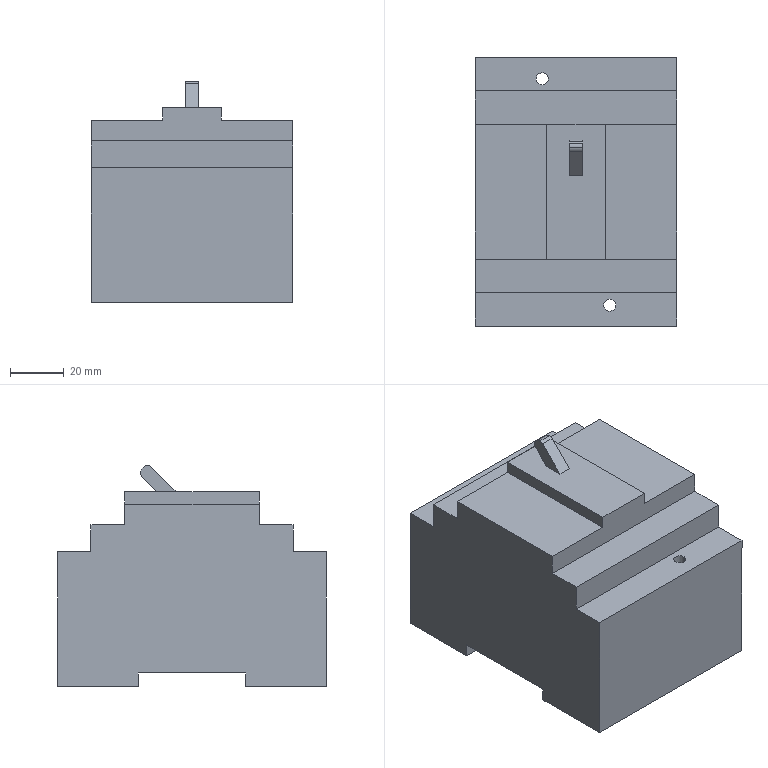Part | SolidWorks | features ICE 5, Extrusion 1, Fillet 1, HoleWzd 1 | 1 solid | 34 faces | box 74.7 x 99.6 x 82.007 mm | volume 445552 mm3 | plane 27 | cylinder 7 | commonest cylinder face diameters 4.5 x4 4 x3
STEP:
#1=CARTESIAN_POINT('',(2.5,16.464,48.157));
#2=VERTEX_POINT('',#1);
#3=CARTESIAN_POINT('',(2.5,15.05,47.571));
#4=VERTEX_POINT('',#3);
#5=CARTESIAN_POINT('',(2.5,16.464,46.157));
#6=DIRECTION('',(1.,0.,0.));
#7=DIRECTION('',(0.,0.,-1.));
#8=AXIS2_PLACEMENT_3D('',#5,#6,#7);
#9=CIRCLE('',#8,2.);
#10=EDGE_CURVE('',#2,#4,#9,.T.);
#11=ORIENTED_EDGE('',*,*,#10,.F.);
#12=CARTESIAN_POINT('',(-2.5,16.464,48.157));
#13=VERTEX_POINT('',#12);
#14=CARTESIAN_POINT('',(2.5,16.464,48.157));
#15=DIRECTION('',(-1.,0.,0.));
#16=VECTOR('',#15,1000.);
#17=LINE('',#14,#16);
#18=EDGE_CURVE('',#2,#13,#17,.T.);
#19=ORIENTED_EDGE('',*,*,#18,.T.);
#20=CARTESIAN_POINT('',(-2.5,15.05,47.571));
#21=VERTEX_POINT('',#20);
#22=CARTESIAN_POINT('',(-2.5,16.464,46.157));
#23=DIRECTION('',(-1.,0.,0.));
#24=DIRECTION('',(0.,0.,-1.));
#25=AXIS2_PLACEMENT_3D('',#22,#23,#24);
#26=CIRCLE('',#25,2.);
#27=EDGE_CURVE('',#21,#13,#26,.T.);
#28=ORIENTED_EDGE('',*,*,#27,.F.);
#29=CARTESIAN_POINT('',(2.5,15.05,47.571));
#30=DIRECTION('',(-1.,0.,0.));
#31=VECTOR('',#30,1000.);
#32=LINE('',#29,#31);
#33=EDGE_CURVE('',#4,#21,#32,.T.);
#34=ORIENTED_EDGE('',*,*,#33,.F.);
#35=EDGE_LOOP('',(#11,#19,#28,#34));
#36=FACE_OUTER_BOUND('',#35,.T.);
#37=CARTESIAN_POINT('',(2.5,16.464,46.157));
#38=DIRECTION('',(-1.,0.,0.));
#39=DIRECTION('',(0.,0.,1.));
#40=AXIS2_PLACEMENT_3D('',#37,#38,#39);
#41=CYLINDRICAL_SURFACE('',#40,2.);
#42=ADVANCED_FACE('',(#36),#41,.T.);
#43=CARTESIAN_POINT('',(-14.75,42.,-33.85));
#44=VERTEX_POINT('',#43);
#45=CARTESIAN_POINT('',(-10.25,42.,-33.85));
#46=VERTEX_POINT('',#45);
#47=CARTESIAN_POINT('',(-12.5,42.,-33.85));
#48=DIRECTION('',(0.,0.,1.));
#49=DIRECTION('',(1.,0.,0.));
#50=AXIS2_PLACEMENT_3D('',#47,#48,#49);
#51=CIRCLE('',#50,2.25);
#52=EDGE_CURVE('',#44,#46,#51,.T.);
#53=ORIENTED_EDGE('',*,*,#52,.F.);
#54=CARTESIAN_POINT('',(-14.75,42.,16.15));
#55=VERTEX_POINT('',#54);
#56=CARTESIAN_POINT('',(-14.75,42.,33.85));
#57=DIRECTION('',(0.,0.,1.));
#58=VECTOR('',#57,1000.);
#59=LINE('',#56,#58);
#60=EDGE_CURVE('',#44,#55,#59,.T.);
#61=ORIENTED_EDGE('',*,*,#60,.T.);
#62=CARTESIAN_POINT('',(-10.25,42.,16.15));
#63=VERTEX_POINT('',#62);
#64=CARTESIAN_POINT('',(-12.5,42.,16.15));
#65=DIRECTION('',(0.,0.,-1.));
#66=DIRECTION('',(1.,0.,0.));
#67=AXIS2_PLACEMENT_3D('',#64,#65,#66);
#68=CIRCLE('',#67,2.25);
#69=EDGE_CURVE('',#63,#55,#68,.T.);
#70=ORIENTED_EDGE('',*,*,#69,.F.);
#71=CARTESIAN_POINT('',(-10.25,42.,33.85));
#72=DIRECTION('',(0.,0.,1.));
#73=VECTOR('',#72,1000.);
#74=LINE('',#71,#73);
#75=EDGE_CURVE('',#46,#63,#74,.T.);
#76=ORIENTED_EDGE('',*,*,#75,.F.);
#77=EDGE_LOOP('',(#53,#61,#70,#76));
#78=FACE_OUTER_BOUND('',#77,.T.);
#79=CARTESIAN_POINT('',(-12.5,42.,33.85));
#80=DIRECTION('',(0.,0.,1.));
#81=DIRECTION('',(1.,0.,0.));
#82=AXIS2_PLACEMENT_3D('',#79,#80,#81);
#83=CYLINDRICAL_SURFACE('',#82,2.25);
#84=ADVANCED_FACE('',(#78),#83,.F.);
#85=CARTESIAN_POINT('',(10.25,-42.,-33.85));
#86=VERTEX_POINT('',#85);
#87=CARTESIAN_POINT('',(14.75,-42.,-33.85));
#88=VERTEX_POINT('',#87);
#89=CARTESIAN_POINT('',(12.5,-42.,-33.85));
#90=DIRECTION('',(0.,0.,1.));
#91=DIRECTION('',(1.,0.,0.));
#92=AXIS2_PLACEMENT_3D('',#89,#90,#91);
#93=CIRCLE('',#92,2.25);
#94=EDGE_CURVE('',#86,#88,#93,.T.);
#95=ORIENTED_EDGE('',*,*,#94,.F.);
#96=CARTESIAN_POINT('',(10.25,-42.,16.15));
#97=VERTEX_POINT('',#96);
#98=CARTESIAN_POINT('',(10.25,-42.,33.85));
#99=DIRECTION('',(0.,0.,1.));
#100=VECTOR('',#99,1000.);
#101=LINE('',#98,#100);
#102=EDGE_CURVE('',#86,#97,#101,.T.);
#103=ORIENTED_EDGE('',*,*,#102,.T.);
#104=CARTESIAN_POINT('',(14.75,-42.,16.15));
#105=VERTEX_POINT('',#104);
#106=CARTESIAN_POINT('',(12.5,-42.,16.15));
#107=DIRECTION('',(0.,0.,-1.));
#108=DIRECTION('',(1.,0.,0.));
#109=AXIS2_PLACEMENT_3D('',#106,#107,#108);
#110=CIRCLE('',#109,2.25);
#111=EDGE_CURVE('',#105,#97,#110,.T.);
#112=ORIENTED_EDGE('',*,*,#111,.F.);
#113=CARTESIAN_POINT('',(14.75,-42.,33.85));
#114=DIRECTION('',(0.,0.,1.));
#115=VECTOR('',#114,1000.);
#116=LINE('',#113,#115);
#117=EDGE_CURVE('',#88,#105,#116,.T.);
#118=ORIENTED_EDGE('',*,*,#117,.F.);
#119=EDGE_LOOP('',(#95,#103,#112,#118));
#120=FACE_OUTER_BOUND('',#119,.T.);
#121=CARTESIAN_POINT('',(12.5,-42.,33.85));
#122=DIRECTION('',(0.,0.,1.));
#123=DIRECTION('',(1.,0.,0.));
#124=AXIS2_PLACEMENT_3D('',#121,#122,#123);
#125=CYLINDRICAL_SURFACE('',#124,2.25);
#126=ADVANCED_FACE('',(#120),#125,.F.);
#127=CARTESIAN_POINT('',(12.5,-42.,-33.85));
#128=DIRECTION('',(0.,0.,1.));
#129=DIRECTION('',(1.,0.,0.));
#130=AXIS2_PLACEMENT_3D('',#127,#128,#129);
#131=CIRCLE('',#130,2.25);
#132=EDGE_CURVE('',#88,#86,#131,.T.);
#133=ORIENTED_EDGE('',*,*,#132,.T.);
#134=ORIENTED_EDGE('',*,*,#94,.T.);
#135=EDGE_LOOP('',(#133,#134));
#136=FACE_BOUND('',#135,.T.);
#137=CARTESIAN_POINT('',(-37.35,-20.,-33.85));
#138=VERTEX_POINT('',#137);
#139=CARTESIAN_POINT('',(-37.35,-49.8,-33.85));
#140=VERTEX_POINT('',#139);
#141=CARTESIAN_POINT('',(-37.35,49.8,-33.85));
#142=DIRECTION('',(0.,-1.,0.));
#143=VECTOR('',#142,1000.);
#144=LINE('',#141,#143);
#145=EDGE_CURVE('',#138,#140,#144,.T.);
#146=ORIENTED_EDGE('',*,*,#145,.F.);
#147=CARTESIAN_POINT('',(37.35,-20.,-33.85));
#148=VERTEX_POINT('',#147);
#149=CARTESIAN_POINT('',(37.35,-20.,-33.85));
#150=DIRECTION('',(1.,0.,0.));
#151=VECTOR('',#150,1000.);
#152=LINE('',#149,#151);
#153=EDGE_CURVE('',#138,#148,#152,.T.);
#154=ORIENTED_EDGE('',*,*,#153,.T.);
#155=CARTESIAN_POINT('',(37.35,-49.8,-33.85));
#156=VERTEX_POINT('',#155);
#157=CARTESIAN_POINT('',(37.35,49.8,-33.85));
#158=DIRECTION('',(0.,1.,0.));
#159=VECTOR('',#158,1000.);
#160=LINE('',#157,#159);
#161=EDGE_CURVE('',#156,#148,#160,.T.);
#162=ORIENTED_EDGE('',*,*,#161,.F.);
#163=CARTESIAN_POINT('',(-37.35,-49.8,-33.85));
#164=DIRECTION('',(1.,0.,0.));
#165=VECTOR('',#164,1000.);
#166=LINE('',#163,#165);
#167=EDGE_CURVE('',#140,#156,#166,.T.);
#168=ORIENTED_EDGE('',*,*,#167,.F.);
#169=EDGE_LOOP('',(#146,#154,#162,#168));
#170=FACE_OUTER_BOUND('',#169,.T.);
#171=CARTESIAN_POINT('',(37.35,-49.8,-33.85));
#172=DIRECTION('',(0.,0.,1.));
#173=DIRECTION('',(1.,0.,0.));
#174=AXIS2_PLACEMENT_3D('',#171,#172,#173);
#175=PLANE('',#174);
#176=ADVANCED_FACE('',(#136,#170),#175,.F.);
#177=CARTESIAN_POINT('',(10.85,-25.,33.85));
#178=VERTEX_POINT('',#177);
#179=CARTESIAN_POINT('',(10.85,25.,33.85));
#180=VERTEX_POINT('',#179);
#181=CARTESIAN_POINT('',(10.85,-25.,33.85));
#182=DIRECTION('',(0.,1.,0.));
#183=VECTOR('',#182,1000.);
#184=LINE('',#181,#183);
#185=EDGE_CURVE('',#178,#180,#184,.T.);
#186=ORIENTED_EDGE('',*,*,#185,.F.);
#187=CARTESIAN_POINT('',(37.35,-25.,33.85));
#188=VERTEX_POINT('',#187);
#189=CARTESIAN_POINT('',(-37.35,-25.,33.85));
#190=DIRECTION('',(-1.,0.,0.));
#191=VECTOR('',#190,1000.);
#192=LINE('',#189,#191);
#193=EDGE_CURVE('',#188,#178,#192,.T.);
#194=ORIENTED_EDGE('',*,*,#193,.F.);
#195=CARTESIAN_POINT('',(37.35,25.,33.85));
#196=VERTEX_POINT('',#195);
#197=CARTESIAN_POINT('',(37.35,49.8,33.85));
#198=DIRECTION('',(0.,1.,0.));
#199=VECTOR('',#198,1000.);
#200=LINE('',#197,#199);
#201=EDGE_CURVE('',#188,#196,#200,.T.);
#202=ORIENTED_EDGE('',*,*,#201,.T.);
#203=CARTESIAN_POINT('',(-37.35,25.,33.85));
#204=DIRECTION('',(1.,0.,0.));
#205=VECTOR('',#204,1000.);
#206=LINE('',#203,#205);
#207=EDGE_CURVE('',#180,#196,#206,.T.);
#208=ORIENTED_EDGE('',*,*,#207,.F.);
#209=EDGE_LOOP('',(#186,#194,#202,#208));
#210=FACE_OUTER_BOUND('',#209,.T.);
#211=CARTESIAN_POINT('',(37.35,-49.8,33.85));
#212=DIRECTION('',(0.,0.,1.));
#213=DIRECTION('',(1.,0.,0.));
#214=AXIS2_PLACEMENT_3D('',#211,#212,#213);
#215=PLANE('',#214);
#216=ADVANCED_FACE('',(#210),#215,.T.);
#217=CARTESIAN_POINT('',(-37.35,-49.8,16.15));
#218=VERTEX_POINT('',#217);
#219=CARTESIAN_POINT('',(37.35,-49.8,16.15));
#220=VERTEX_POINT('',#219);
#221=CARTESIAN_POINT('',(-37.35,-49.8,16.15));
#222=DIRECTION('',(1.,0.,0.));
#223=VECTOR('',#222,1000.);
#224=LINE('',#221,#223);
#225=EDGE_CURVE('',#218,#220,#224,.T.);
#226=ORIENTED_EDGE('',*,*,#225,.F.);
#227=CARTESIAN_POINT('',(-37.35,-49.8,33.85));
#228=DIRECTION('',(0.,0.,-1.));
#229=VECTOR('',#228,1000.);
#230=LINE('',#227,#229);
#231=EDGE_CURVE('',#218,#140,#230,.T.);
#232=ORIENTED_EDGE('',*,*,#231,.T.);
#233=ORIENTED_EDGE('',*,*,#167,.T.);
#234=CARTESIAN_POINT('',(37.35,-49.8,33.85));
#235=DIRECTION('',(0.,0.,-1.));
#236=VECTOR('',#235,1000.);
#237=LINE('',#234,#236);
#238=EDGE_CURVE('',#220,#156,#237,.T.);
#239=ORIENTED_EDGE('',*,*,#238,.F.);
#240=EDGE_LOOP('',(#226,#232,#233,#239));
#241=FACE_OUTER_BOUND('',#240,.T.);
#242=CARTESIAN_POINT('',(-37.35,-49.8,33.85));
#243=DIRECTION('',(0.,1.,0.));
#244=DIRECTION('',(0.,0.,1.));
#245=AXIS2_PLACEMENT_3D('',#242,#243,#244);
#246=PLANE('',#245);
#247=ADVANCED_FACE('',(#241),#246,.F.);
#248=ORIENTED_EDGE('',*,*,#102,.F.);
#249=ORIENTED_EDGE('',*,*,#132,.F.);
#250=ORIENTED_EDGE('',*,*,#117,.T.);
#251=CARTESIAN_POINT('',(12.5,-42.,16.15));
#252=DIRECTION('',(0.,0.,-1.));
#253=DIRECTION('',(1.,0.,0.));
#254=AXIS2_PLACEMENT_3D('',#251,#252,#253);
#255=CIRCLE('',#254,2.25);
#256=EDGE_CURVE('',#97,#105,#255,.T.);
#257=ORIENTED_EDGE('',*,*,#256,.F.);
#258=EDGE_LOOP('',(#248,#249,#250,#257));
#259=FACE_OUTER_BOUND('',#258,.T.);
#260=CARTESIAN_POINT('',(12.5,-42.,33.85));
#261=DIRECTION('',(0.,0.,1.));
#262=DIRECTION('',(1.,0.,0.));
#263=AXIS2_PLACEMENT_3D('',#260,#261,#262);
#264=CYLINDRICAL_SURFACE('',#263,2.25);
#265=ADVANCED_FACE('',(#259),#264,.F.);
#266=CARTESIAN_POINT('',(37.35,49.8,16.15));
#267=VERTEX_POINT('',#266);
#268=CARTESIAN_POINT('',(-37.35,49.8,16.15));
#269=VERTEX_POINT('',#268);
#270=CARTESIAN_POINT('',(-37.35,49.8,16.15));
#271=DIRECTION('',(-1.,0.,0.));
#272=VECTOR('',#271,1000.);
#273=LINE('',#270,#272);
#274=EDGE_CURVE('',#267,#269,#273,.T.);
#275=ORIENTED_EDGE('',*,*,#274,.F.);
#276=CARTESIAN_POINT('',(37.35,49.8,-33.85));
#277=VERTEX_POINT('',#276);
#278=CARTESIAN_POINT('',(37.35,49.8,33.85));
#279=DIRECTION('',(0.,0.,-1.));
#280=VECTOR('',#279,1000.);
#281=LINE('',#278,#280);
#282=EDGE_CURVE('',#267,#277,#281,.T.);
#283=ORIENTED_EDGE('',*,*,#282,.T.);
#284=CARTESIAN_POINT('',(-37.35,49.8,-33.85));
#285=VERTEX_POINT('',#284);
#286=CARTESIAN_POINT('',(-37.35,49.8,-33.85));
#287=DIRECTION('',(-1.,0.,0.));
#288=VECTOR('',#287,1000.);
#289=LINE('',#286,#288);
#290=EDGE_CURVE('',#277,#285,#289,.T.);
#291=ORIENTED_EDGE('',*,*,#290,.T.);
#292=CARTESIAN_POINT('',(-37.35,49.8,33.85));
#293=DIRECTION('',(0.,0.,-1.));
#294=VECTOR('',#293,1000.);
#295=LINE('',#292,#294);
#296=EDGE_CURVE('',#269,#285,#295,.T.);
#297=ORIENTED_EDGE('',*,*,#296,.F.);
#298=EDGE_LOOP('',(#275,#283,#291,#297));
#299=FACE_OUTER_BOUND('',#298,.T.);
#300=CARTESIAN_POINT('',(-37.35,49.8,33.85));
#301=DIRECTION('',(0.,-1.,0.));
#302=DIRECTION('',(0.,0.,-1.));
#303=AXIS2_PLACEMENT_3D('',#300,#301,#302);
#304=PLANE('',#303);
#305=ADVANCED_FACE('',(#299),#304,.F.);
#306=ORIENTED_EDGE('',*,*,#60,.F.);
#307=CARTESIAN_POINT('',(-12.5,42.,-33.85));
#308=DIRECTION('',(0.,0.,1.));
#309=DIRECTION('',(1.,0.,0.));
#310=AXIS2_PLACEMENT_3D('',#307,#308,#309);
#311=CIRCLE('',#310,2.25);
#312=EDGE_CURVE('',#46,#44,#311,.T.);
#313=ORIENTED_EDGE('',*,*,#312,.F.);
#314=ORIENTED_EDGE('',*,*,#75,.T.);
#315=CARTESIAN_POINT('',(-12.5,42.,16.15));
#316=DIRECTION('',(0.,0.,-1.));
#317=DIRECTION('',(1.,0.,0.));
#318=AXIS2_PLACEMENT_3D('',#315,#316,#317);
#319=CIRCLE('',#318,2.25);
#320=EDGE_CURVE('',#55,#63,#319,.T.);
#321=ORIENTED_EDGE('',*,*,#320,.F.);
#322=EDGE_LOOP('',(#306,#313,#314,#321));
#323=FACE_OUTER_BOUND('',#322,.T.);
#324=CARTESIAN_POINT('',(-12.5,42.,33.85));
#325=DIRECTION('',(0.,0.,1.));
#326=DIRECTION('',(1.,0.,0.));
#327=AXIS2_PLACEMENT_3D('',#324,#325,#326);
#328=CYLINDRICAL_SURFACE('',#327,2.25);
#329=ADVANCED_FACE('',(#323),#328,.F.);
#330=ORIENTED_EDGE('',*,*,#161,.T.);
#331=CARTESIAN_POINT('',(37.35,-20.,-28.85));
#332=VERTEX_POINT('',#331);
#333=CARTESIAN_POINT('',(37.35,-20.,-33.85));
#334=DIRECTION('',(0.,0.,-1.));
#335=VECTOR('',#334,1000.);
#336=LINE('',#333,#335);
#337=EDGE_CURVE('',#332,#148,#336,.T.);
#338=ORIENTED_EDGE('',*,*,#337,.F.);
#339=CARTESIAN_POINT('',(37.35,20.,-28.85));
#340=VERTEX_POINT('',#339);
#341=CARTESIAN_POINT('',(37.35,-20.,-28.85));
#342=DIRECTION('',(0.,-1.,0.));
#343=VECTOR('',#342,1000.);
#344=LINE('',#341,#343);
#345=EDGE_CURVE('',#340,#332,#344,.T.);
#346=ORIENTED_EDGE('',*,*,#345,.F.);
#347=CARTESIAN_POINT('',(37.35,20.,-33.85));
#348=VERTEX_POINT('',#347);
#349=CARTESIAN_POINT('',(37.35,20.,-33.85));
#350=DIRECTION('',(0.,0.,1.));
#351=VECTOR('',#350,1000.);
#352=LINE('',#349,#351);
#353=EDGE_CURVE('',#348,#340,#352,.T.);
#354=ORIENTED_EDGE('',*,*,#353,.F.);
#355=CARTESIAN_POINT('',(37.35,49.8,-33.85));
#356=DIRECTION('',(0.,1.,0.));
#357=VECTOR('',#356,1000.);
#358=LINE('',#355,#357);
#359=EDGE_CURVE('',#348,#277,#358,.T.);
#360=ORIENTED_EDGE('',*,*,#359,.T.);
#361=ORIENTED_EDGE('',*,*,#282,.F.);
#362=CARTESIAN_POINT('',(37.35,37.5,16.15));
#363=VERTEX_POINT('',#362);
#364=CARTESIAN_POINT('',(37.35,49.8,16.15));
#365=DIRECTION('',(0.,1.,0.));
#366=VECTOR('',#365,1000.);
#367=LINE('',#364,#366);
#368=EDGE_CURVE('',#363,#267,#367,.T.);
#369=ORIENTED_EDGE('',*,*,#368,.F.);
#370=CARTESIAN_POINT('',(37.35,37.5,26.15));
#371=VERTEX_POINT('',#370);
#372=CARTESIAN_POINT('',(37.35,37.5,16.15));
#373=DIRECTION('',(0.,0.,1.));
#374=VECTOR('',#373,1000.);
#375=LINE('',#372,#374);
#376=EDGE_CURVE('',#363,#371,#375,.T.);
#377=ORIENTED_EDGE('',*,*,#376,.T.);
#378=CARTESIAN_POINT('',(37.35,25.,26.15));
#379=VERTEX_POINT('',#378);
#380=CARTESIAN_POINT('',(37.35,37.5,26.15));
#381=DIRECTION('',(0.,1.,0.));
#382=VECTOR('',#381,1000.);
#383=LINE('',#380,#382);
#384=EDGE_CURVE('',#379,#371,#383,.T.);
#385=ORIENTED_EDGE('',*,*,#384,.F.);
#386=CARTESIAN_POINT('',(37.35,25.,26.15));
#387=DIRECTION('',(0.,0.,1.));
#388=VECTOR('',#387,1000.);
#389=LINE('',#386,#388);
#390=EDGE_CURVE('',#379,#196,#389,.T.);
#391=ORIENTED_EDGE('',*,*,#390,.T.);
#392=ORIENTED_EDGE('',*,*,#201,.F.);
#393=CARTESIAN_POINT('',(37.35,-25.,26.15));
#394=VERTEX_POINT('',#393);
#395=CARTESIAN_POINT('',(37.35,-25.,26.15));
#396=DIRECTION('',(0.,0.,1.));
#397=VECTOR('',#396,1000.);
#398=LINE('',#395,#397);
#399=EDGE_CURVE('',#394,#188,#398,.T.);
#400=ORIENTED_EDGE('',*,*,#399,.F.);
#401=CARTESIAN_POINT('',(37.35,-37.5,26.15));
#402=VERTEX_POINT('',#401);
#403=CARTESIAN_POINT('',(37.35,-37.5,26.15));
#404=DIRECTION('',(0.,1.,0.));
#405=VECTOR('',#404,1000.);
#406=LINE('',#403,#405);
#407=EDGE_CURVE('',#402,#394,#406,.T.);
#408=ORIENTED_EDGE('',*,*,#407,.F.);
#409=CARTESIAN_POINT('',(37.35,-37.5,16.15));
#410=VERTEX_POINT('',#409);
#411=CARTESIAN_POINT('',(37.35,-37.5,16.15));
#412=DIRECTION('',(0.,0.,1.));
#413=VECTOR('',#412,1000.);
#414=LINE('',#411,#413);
#415=EDGE_CURVE('',#410,#402,#414,.T.);
#416=ORIENTED_EDGE('',*,*,#415,.F.);
#417=CARTESIAN_POINT('',(37.35,-49.8,16.15));
#418=DIRECTION('',(0.,1.,0.));
#419=VECTOR('',#418,1000.);
#420=LINE('',#417,#419);
#421=EDGE_CURVE('',#220,#410,#420,.T.);
#422=ORIENTED_EDGE('',*,*,#421,.F.);
#423=ORIENTED_EDGE('',*,*,#238,.T.);
#424=EDGE_LOOP('',(#330,#338,#346,#354,#360,#361,#369,#377,#385,#391,#392,#400,#408,#416,#422,#423));
#425=FACE_OUTER_BOUND('',#424,.T.);
#426=CARTESIAN_POINT('',(37.35,49.8,33.85));
#427=DIRECTION('',(-1.,0.,0.));
#428=DIRECTION('',(0.,-1.,0.));
#429=AXIS2_PLACEMENT_3D('',#426,#427,#428);
#430=PLANE('',#429);
#431=ADVANCED_FACE('',(#425),#430,.F.);
#432=CARTESIAN_POINT('',(-37.35,20.,-28.85));
#433=VERTEX_POINT('',#432);
#434=CARTESIAN_POINT('',(-37.35,-20.,-28.85));
#435=VERTEX_POINT('',#434);
#436=CARTESIAN_POINT('',(-37.35,49.8,-28.85));
#437=DIRECTION('',(0.,-1.,0.));
#438=VECTOR('',#437,1000.);
#439=LINE('',#436,#438);
#440=EDGE_CURVE('',#433,#435,#439,.T.);
#441=ORIENTED_EDGE('',*,*,#440,.T.);
#442=CARTESIAN_POINT('',(-37.35,-20.,33.85));
#443=DIRECTION('',(0.,0.,-1.));
#444=VECTOR('',#443,1000.);
#445=LINE('',#442,#444);
#446=EDGE_CURVE('',#435,#138,#445,.T.);
#447=ORIENTED_EDGE('',*,*,#446,.T.);
#448=ORIENTED_EDGE('',*,*,#145,.T.);
#449=ORIENTED_EDGE('',*,*,#231,.F.);
#450=CARTESIAN_POINT('',(-37.35,-37.5,16.15));
#451=VERTEX_POINT('',#450);
#452=CARTESIAN_POINT('',(-37.35,-49.8,16.15));
#453=DIRECTION('',(0.,-1.,0.));
#454=VECTOR('',#453,1000.);
#455=LINE('',#452,#454);
#456=EDGE_CURVE('',#451,#218,#455,.T.);
#457=ORIENTED_EDGE('',*,*,#456,.F.);
#458=CARTESIAN_POINT('',(-37.35,-37.5,26.15));
#459=VERTEX_POINT('',#458);
#460=CARTESIAN_POINT('',(-37.35,-37.5,16.15));
#461=DIRECTION('',(0.,0.,1.));
#462=VECTOR('',#461,1000.);
#463=LINE('',#460,#462);
#464=EDGE_CURVE('',#451,#459,#463,.T.);
#465=ORIENTED_EDGE('',*,*,#464,.T.);
#466=CARTESIAN_POINT('',(-37.35,-25.,26.15));
#467=VERTEX_POINT('',#466);
#468=CARTESIAN_POINT('',(-37.35,-37.5,26.15));
#469=DIRECTION('',(0.,-1.,0.));
#470=VECTOR('',#469,1000.);
#471=LINE('',#468,#470);
#472=EDGE_CURVE('',#467,#459,#471,.T.);
#473=ORIENTED_EDGE('',*,*,#472,.F.);
#474=CARTESIAN_POINT('',(-37.35,-25.,33.85));
#475=VERTEX_POINT('',#474);
#476=CARTESIAN_POINT('',(-37.35,-25.,26.15));
#477=DIRECTION('',(0.,0.,1.));
#478=VECTOR('',#477,1000.);
#479=LINE('',#476,#478);
#480=EDGE_CURVE('',#467,#475,#479,.T.);
#481=ORIENTED_EDGE('',*,*,#480,.T.);
#482=CARTESIAN_POINT('',(-37.35,25.,33.85));
#483=VERTEX_POINT('',#482);
#484=CARTESIAN_POINT('',(-37.35,49.8,33.85));
#485=DIRECTION('',(0.,-1.,0.));
#486=VECTOR('',#485,1000.);
#487=LINE('',#484,#486);
#488=EDGE_CURVE('',#483,#475,#487,.T.);
#489=ORIENTED_EDGE('',*,*,#488,.F.);
#490=CARTESIAN_POINT('',(-37.35,25.,26.15));
#491=VERTEX_POINT('',#490);
#492=CARTESIAN_POINT('',(-37.35,25.,26.15));
#493=DIRECTION('',(0.,0.,1.));
#494=VECTOR('',#493,1000.);
#495=LINE('',#492,#494);
#496=EDGE_CURVE('',#491,#483,#495,.T.);
#497=ORIENTED_EDGE('',*,*,#496,.F.);
#498=CARTESIAN_POINT('',(-37.35,37.5,26.15));
#499=VERTEX_POINT('',#498);
#500=CARTESIAN_POINT('',(-37.35,37.5,26.15));
#501=DIRECTION('',(0.,-1.,0.));
#502=VECTOR('',#501,1000.);
#503=LINE('',#500,#502);
#504=EDGE_CURVE('',#499,#491,#503,.T.);
#505=ORIENTED_EDGE('',*,*,#504,.F.);
#506=CARTESIAN_POINT('',(-37.35,37.5,16.15));
#507=VERTEX_POINT('',#506);
#508=CARTESIAN_POINT('',(-37.35,37.5,16.15));
#509=DIRECTION('',(0.,0.,1.));
#510=VECTOR('',#509,1000.);
#511=LINE('',#508,#510);
#512=EDGE_CURVE('',#507,#499,#511,.T.);
#513=ORIENTED_EDGE('',*,*,#512,.F.);
#514=CARTESIAN_POINT('',(-37.35,49.8,16.15));
#515=DIRECTION('',(0.,-1.,0.));
#516=VECTOR('',#515,1000.);
#517=LINE('',#514,#516);
#518=EDGE_CURVE('',#269,#507,#517,.T.);
#519=ORIENTED_EDGE('',*,*,#518,.F.);
#520=ORIENTED_EDGE('',*,*,#296,.T.);
#521=CARTESIAN_POINT('',(-37.35,20.,-33.85));
#522=VERTEX_POINT('',#521);
#523=CARTESIAN_POINT('',(-37.35,49.8,-33.85));
#524=DIRECTION('',(0.,-1.,0.));
#525=VECTOR('',#524,1000.);
#526=LINE('',#523,#525);
#527=EDGE_CURVE('',#285,#522,#526,.T.);
#528=ORIENTED_EDGE('',*,*,#527,.T.);
#529=CARTESIAN_POINT('',(-37.35,20.,33.85));
#530=DIRECTION('',(0.,0.,1.));
#531=VECTOR('',#530,1000.);
#532=LINE('',#529,#531);
#533=EDGE_CURVE('',#522,#433,#532,.T.);
#534=ORIENTED_EDGE('',*,*,#533,.T.);
#535=EDGE_LOOP('',(#441,#447,#448,#449,#457,#465,#473,#481,#489,#497,#505,#513,#519,#520,#528,#534));
#536=FACE_OUTER_BOUND('',#535,.T.);
#537=CARTESIAN_POINT('',(-37.35,49.8,33.85));
#538=DIRECTION('',(1.,0.,0.));
#539=DIRECTION('',(0.,1.,0.));
#540=AXIS2_PLACEMENT_3D('',#537,#538,#539);
#541=PLANE('',#540);
#542=ADVANCED_FACE('',(#536),#541,.F.);
#543=CARTESIAN_POINT('',(-10.85,25.,33.85));
#544=VERTEX_POINT('',#543);
#545=CARTESIAN_POINT('',(-10.85,-25.,33.85));
#546=VERTEX_POINT('',#545);
#547=CARTESIAN_POINT('',(-10.85,-25.,33.85));
#548=DIRECTION('',(0.,-1.,0.));
#549=VECTOR('',#548,1000.);
#550=LINE('',#547,#549);
#551=EDGE_CURVE('',#544,#546,#550,.T.);
#552=ORIENTED_EDGE('',*,*,#551,.F.);
#553=CARTESIAN_POINT('',(-37.35,25.,33.85));
#554=DIRECTION('',(1.,0.,0.));
#555=VECTOR('',#554,1000.);
#556=LINE('',#553,#555);
#557=EDGE_CURVE('',#483,#544,#556,.T.);
#558=ORIENTED_EDGE('',*,*,#557,.F.);
#559=ORIENTED_EDGE('',*,*,#488,.T.);
#560=CARTESIAN_POINT('',(-37.35,-25.,33.85));
#561=DIRECTION('',(-1.,0.,0.));
#562=VECTOR('',#561,1000.);
#563=LINE('',#560,#562);
#564=EDGE_CURVE('',#546,#475,#563,.T.);
#565=ORIENTED_EDGE('',*,*,#564,.F.);
#566=EDGE_LOOP('',(#552,#558,#559,#565));
#567=FACE_OUTER_BOUND('',#566,.T.);
#568=CARTESIAN_POINT('',(37.35,-49.8,33.85));
#569=DIRECTION('',(0.,0.,1.));
#570=DIRECTION('',(1.,0.,0.));
#571=AXIS2_PLACEMENT_3D('',#568,#569,#570);
#572=PLANE('',#571);
#573=ADVANCED_FACE('',(#567),#572,.T.);
#574=ORIENTED_EDGE('',*,*,#312,.T.);
#575=ORIENTED_EDGE('',*,*,#52,.T.);
#576=EDGE_LOOP('',(#574,#575));
#577=FACE_BOUND('',#576,.T.);
#578=ORIENTED_EDGE('',*,*,#359,.F.);
#579=CARTESIAN_POINT('',(37.35,20.,-33.85));
#580=DIRECTION('',(-1.,0.,0.));
#581=VECTOR('',#580,1000.);
#582=LINE('',#579,#581);
#583=EDGE_CURVE('',#348,#522,#582,.T.);
#584=ORIENTED_EDGE('',*,*,#583,.T.);
#585=ORIENTED_EDGE('',*,*,#527,.F.);
#586=ORIENTED_EDGE('',*,*,#290,.F.);
#587=EDGE_LOOP('',(#578,#584,#585,#586));
#588=FACE_OUTER_BOUND('',#587,.T.);
#589=CARTESIAN_POINT('',(37.35,-49.8,-33.85));
#590=DIRECTION('',(0.,0.,1.));
#591=DIRECTION('',(1.,0.,0.));
#592=AXIS2_PLACEMENT_3D('',#589,#590,#591);
#593=PLANE('',#592);
#594=ADVANCED_FACE('',(#577,#588),#593,.F.);
#595=ORIENTED_EDGE('',*,*,#518,.T.);
#596=CARTESIAN_POINT('',(-37.35,37.5,16.15));
#597=DIRECTION('',(1.,0.,0.));
#598=VECTOR('',#597,1000.);
#599=LINE('',#596,#598);
#600=EDGE_CURVE('',#507,#363,#599,.T.);
#601=ORIENTED_EDGE('',*,*,#600,.T.);
#602=ORIENTED_EDGE('',*,*,#368,.T.);
#603=ORIENTED_EDGE('',*,*,#274,.T.);
#604=EDGE_LOOP('',(#595,#601,#602,#603));
#605=FACE_OUTER_BOUND('',#604,.T.);
#606=ORIENTED_EDGE('',*,*,#69,.T.);
#607=ORIENTED_EDGE('',*,*,#320,.T.);
#608=EDGE_LOOP('',(#606,#607));
#609=FACE_BOUND('',#608,.T.);
#610=CARTESIAN_POINT('',(-37.35,37.5,16.15));
#611=DIRECTION('',(0.,0.,1.));
#612=DIRECTION('',(1.,0.,0.));
#613=AXIS2_PLACEMENT_3D('',#610,#611,#612);
#614=PLANE('',#613);
#615=ADVANCED_FACE('',(#605,#609),#614,.T.);
#616=ORIENTED_EDGE('',*,*,#512,.T.);
#617=CARTESIAN_POINT('',(-37.35,37.5,26.15));
#618=DIRECTION('',(-1.,0.,0.));
#619=VECTOR('',#618,1000.);
#620=LINE('',#617,#619);
#621=EDGE_CURVE('',#371,#499,#620,.T.);
#622=ORIENTED_EDGE('',*,*,#621,.F.);
#623=ORIENTED_EDGE('',*,*,#376,.F.);
#624=ORIENTED_EDGE('',*,*,#600,.F.);
#625=EDGE_LOOP('',(#616,#622,#623,#624));
#626=FACE_OUTER_BOUND('',#625,.T.);
#627=CARTESIAN_POINT('',(-37.35,37.5,16.15));
#628=DIRECTION('',(0.,-1.,0.));
#629=DIRECTION('',(0.,0.,-1.));
#630=AXIS2_PLACEMENT_3D('',#627,#628,#629);
#631=PLANE('',#630);
#632=ADVANCED_FACE('',(#626),#631,.F.);
#633=ORIENTED_EDGE('',*,*,#225,.T.);
#634=ORIENTED_EDGE('',*,*,#421,.T.);
#635=CARTESIAN_POINT('',(-37.35,-37.5,16.15));
#636=DIRECTION('',(-1.,0.,0.));
#637=VECTOR('',#636,1000.);
#638=LINE('',#635,#637);
#639=EDGE_CURVE('',#410,#451,#638,.T.);
#640=ORIENTED_EDGE('',*,*,#639,.T.);
#641=ORIENTED_EDGE('',*,*,#456,.T.);
#642=EDGE_LOOP('',(#633,#634,#640,#641));
#643=FACE_OUTER_BOUND('',#642,.T.);
#644=ORIENTED_EDGE('',*,*,#111,.T.);
#645=ORIENTED_EDGE('',*,*,#256,.T.);
#646=EDGE_LOOP('',(#644,#645));
#647=FACE_BOUND('',#646,.T.);
#648=CARTESIAN_POINT('',(37.35,-49.8,16.15));
#649=DIRECTION('',(0.,0.,1.));
#650=DIRECTION('',(1.,0.,0.));
#651=AXIS2_PLACEMENT_3D('',#648,#649,#650);
#652=PLANE('',#651);
#653=ADVANCED_FACE('',(#643,#647),#652,.T.);
#654=ORIENTED_EDGE('',*,*,#415,.T.);
#655=CARTESIAN_POINT('',(-37.35,-37.5,26.15));
#656=DIRECTION('',(1.,0.,0.));
#657=VECTOR('',#656,1000.);
#658=LINE('',#655,#657);
#659=EDGE_CURVE('',#459,#402,#658,.T.);
#660=ORIENTED_EDGE('',*,*,#659,.F.);
#661=ORIENTED_EDGE('',*,*,#464,.F.);
#662=ORIENTED_EDGE('',*,*,#639,.F.);
#663=EDGE_LOOP('',(#654,#660,#661,#662));
#664=FACE_OUTER_BOUND('',#663,.T.);
#665=CARTESIAN_POINT('',(-37.35,-37.5,16.15));
#666=DIRECTION('',(0.,1.,0.));
#667=DIRECTION('',(0.,0.,1.));
#668=AXIS2_PLACEMENT_3D('',#665,#666,#667);
#669=PLANE('',#668);
#670=ADVANCED_FACE('',(#664),#669,.F.);
#671=ORIENTED_EDGE('',*,*,#193,.T.);
#672=CARTESIAN_POINT('',(10.85,-25.,38.45));
#673=VERTEX_POINT('',#672);
#674=CARTESIAN_POINT('',(10.85,-25.,38.45));
#675=DIRECTION('',(0.,0.,-1.));
#676=VECTOR('',#675,1000.);
#677=LINE('',#674,#676);
#678=EDGE_CURVE('',#673,#178,#677,.T.);
#679=ORIENTED_EDGE('',*,*,#678,.F.);
#680=CARTESIAN_POINT('',(-10.85,-25.,38.45));
#681=VERTEX_POINT('',#680);
#682=CARTESIAN_POINT('',(-10.85,-25.,38.45));
#683=DIRECTION('',(1.,0.,0.));
#684=VECTOR('',#683,1000.);
#685=LINE('',#682,#684);
#686=EDGE_CURVE('',#681,#673,#685,.T.);
#687=ORIENTED_EDGE('',*,*,#686,.F.);
#688=CARTESIAN_POINT('',(-10.85,-25.,38.45));
#689=DIRECTION('',(0.,0.,-1.));
#690=VECTOR('',#689,1000.);
#691=LINE('',#688,#690);
#692=EDGE_CURVE('',#681,#546,#691,.T.);
#693=ORIENTED_EDGE('',*,*,#692,.T.);
#694=ORIENTED_EDGE('',*,*,#564,.T.);
#695=ORIENTED_EDGE('',*,*,#480,.F.);
#696=CARTESIAN_POINT('',(-37.35,-25.,26.15));
#697=DIRECTION('',(-1.,0.,0.));
#698=VECTOR('',#697,1000.);
#699=LINE('',#696,#698);
#700=EDGE_CURVE('',#394,#467,#699,.T.);
#701=ORIENTED_EDGE('',*,*,#700,.F.);
#702=ORIENTED_EDGE('',*,*,#399,.T.);
#703=EDGE_LOOP('',(#671,#679,#687,#693,#694,#695,#701,#702));
#704=FACE_OUTER_BOUND('',#703,.T.);
#705=CARTESIAN_POINT('',(-37.35,-25.,26.15));
#706=DIRECTION('',(0.,1.,0.));
#707=DIRECTION('',(0.,0.,1.));
#708=AXIS2_PLACEMENT_3D('',#705,#706,#707);
#709=PLANE('',#708);
#710=ADVANCED_FACE('',(#704),#709,.F.);
#711=ORIENTED_EDGE('',*,*,#472,.T.);
#712=ORIENTED_EDGE('',*,*,#659,.T.);
#713=ORIENTED_EDGE('',*,*,#407,.T.);
#714=ORIENTED_EDGE('',*,*,#700,.T.);
#715=EDGE_LOOP('',(#711,#712,#713,#714));
#716=FACE_OUTER_BOUND('',#715,.T.);
#717=CARTESIAN_POINT('',(-37.35,-25.,26.15));
#718=DIRECTION('',(0.,0.,-1.));
#719=DIRECTION('',(-1.,0.,0.));
#720=AXIS2_PLACEMENT_3D('',#717,#718,#719);
#721=PLANE('',#720);
#722=ADVANCED_FACE('',(#716),#721,.F.);
#723=ORIENTED_EDGE('',*,*,#557,.T.);
#724=CARTESIAN_POINT('',(-10.85,25.,38.45));
#725=VERTEX_POINT('',#724);
#726=CARTESIAN_POINT('',(-10.85,25.,38.45));
#727=DIRECTION('',(0.,0.,-1.));
#728=VECTOR('',#727,1000.);
#729=LINE('',#726,#728);
#730=EDGE_CURVE('',#725,#544,#729,.T.);
#731=ORIENTED_EDGE('',*,*,#730,.F.);
#732=CARTESIAN_POINT('',(10.85,25.,38.45));
#733=VERTEX_POINT('',#732);
#734=CARTESIAN_POINT('',(-10.85,25.,38.45));
#735=DIRECTION('',(-1.,0.,0.));
#736=VECTOR('',#735,1000.);
#737=LINE('',#734,#736);
#738=EDGE_CURVE('',#733,#725,#737,.T.);
#739=ORIENTED_EDGE('',*,*,#738,.F.);
#740=CARTESIAN_POINT('',(10.85,25.,38.45));
#741=DIRECTION('',(0.,0.,-1.));
#742=VECTOR('',#741,1000.);
#743=LINE('',#740,#742);
#744=EDGE_CURVE('',#733,#180,#743,.T.);
#745=ORIENTED_EDGE('',*,*,#744,.T.);
#746=ORIENTED_EDGE('',*,*,#207,.T.);
#747=ORIENTED_EDGE('',*,*,#390,.F.);
#748=CARTESIAN_POINT('',(-37.35,25.,26.15));
#749=DIRECTION('',(1.,0.,0.));
#750=VECTOR('',#749,1000.);
#751=LINE('',#748,#750);
#752=EDGE_CURVE('',#491,#379,#751,.T.);
#753=ORIENTED_EDGE('',*,*,#752,.F.);
#754=ORIENTED_EDGE('',*,*,#496,.T.);
#755=EDGE_LOOP('',(#723,#731,#739,#745,#746,#747,#753,#754));
#756=FACE_OUTER_BOUND('',#755,.T.);
#757=CARTESIAN_POINT('',(-37.35,25.,26.15));
#758=DIRECTION('',(0.,-1.,0.));
#759=DIRECTION('',(1.,0.,0.));
#760=AXIS2_PLACEMENT_3D('',#757,#758,#759);
#761=PLANE('',#760);
#762=ADVANCED_FACE('',(#756),#761,.F.);
#763=ORIENTED_EDGE('',*,*,#621,.T.);
#764=ORIENTED_EDGE('',*,*,#504,.T.);
#765=ORIENTED_EDGE('',*,*,#752,.T.);
#766=ORIENTED_EDGE('',*,*,#384,.T.);
#767=EDGE_LOOP('',(#763,#764,#765,#766));
#768=FACE_OUTER_BOUND('',#767,.T.);
#769=CARTESIAN_POINT('',(37.35,37.5,26.15));
#770=DIRECTION('',(0.,0.,-1.));
#771=DIRECTION('',(-1.,0.,0.));
#772=AXIS2_PLACEMENT_3D('',#769,#770,#771);
#773=PLANE('',#772);
#774=ADVANCED_FACE('',(#768),#773,.F.);
#775=ORIENTED_EDGE('',*,*,#185,.T.);
#776=ORIENTED_EDGE('',*,*,#744,.F.);
#777=CARTESIAN_POINT('',(10.85,-25.,38.45));
#778=DIRECTION('',(0.,1.,0.));
#779=VECTOR('',#778,1000.);
#780=LINE('',#777,#779);
#781=EDGE_CURVE('',#673,#733,#780,.T.);
#782=ORIENTED_EDGE('',*,*,#781,.F.);
#783=ORIENTED_EDGE('',*,*,#678,.T.);
#784=EDGE_LOOP('',(#775,#776,#782,#783));
#785=FACE_OUTER_BOUND('',#784,.T.);
#786=CARTESIAN_POINT('',(10.85,-25.,38.45));
#787=DIRECTION('',(-1.,0.,0.));
#788=DIRECTION('',(0.,0.,1.));
#789=AXIS2_PLACEMENT_3D('',#786,#787,#788);
#790=PLANE('',#789);
#791=ADVANCED_FACE('',(#785),#790,.F.);
#792=ORIENTED_EDGE('',*,*,#551,.T.);
#793=ORIENTED_EDGE('',*,*,#692,.F.);
#794=CARTESIAN_POINT('',(-10.85,-25.,38.45));
#795=DIRECTION('',(0.,-1.,0.));
#796=VECTOR('',#795,1000.);
#797=LINE('',#794,#796);
#798=EDGE_CURVE('',#725,#681,#797,.T.);
#799=ORIENTED_EDGE('',*,*,#798,.F.);
#800=ORIENTED_EDGE('',*,*,#730,.T.);
#801=EDGE_LOOP('',(#792,#793,#799,#800));
#802=FACE_OUTER_BOUND('',#801,.T.);
#803=CARTESIAN_POINT('',(-10.85,-25.,38.45));
#804=DIRECTION('',(1.,0.,0.));
#805=DIRECTION('',(0.,0.,-1.));
#806=AXIS2_PLACEMENT_3D('',#803,#804,#805);
#807=PLANE('',#806);
#808=ADVANCED_FACE('',(#802),#807,.F.);
#809=CARTESIAN_POINT('',(2.5,13.,38.45));
#810=VERTEX_POINT('',#809);
#811=CARTESIAN_POINT('',(-2.5,13.,38.45));
#812=VERTEX_POINT('',#811);
#813=CARTESIAN_POINT('',(2.5,13.,38.45));
#814=DIRECTION('',(-1.,0.,0.));
#815=VECTOR('',#814,1000.);
#816=LINE('',#813,#815);
#817=EDGE_CURVE('',#810,#812,#816,.T.);
#818=ORIENTED_EDGE('',*,*,#817,.F.);
#819=CARTESIAN_POINT('',(2.5,5.929,38.45));
#820=VERTEX_POINT('',#819);
#821=CARTESIAN_POINT('',(2.5,13.,38.45));
#822=DIRECTION('',(0.,1.,0.));
#823=VECTOR('',#822,1000.);
#824=LINE('',#821,#823);
#825=EDGE_CURVE('',#820,#810,#824,.T.);
#826=ORIENTED_EDGE('',*,*,#825,.F.);
#827=CARTESIAN_POINT('',(-2.5,5.929,38.45));
#828=VERTEX_POINT('',#827);
#829=CARTESIAN_POINT('',(2.5,5.929,38.45));
#830=DIRECTION('',(-1.,0.,0.));
#831=VECTOR('',#830,1000.);
#832=LINE('',#829,#831);
#833=EDGE_CURVE('',#820,#828,#832,.T.);
#834=ORIENTED_EDGE('',*,*,#833,.T.);
#835=CARTESIAN_POINT('',(-2.5,13.,38.45));
#836=DIRECTION('',(0.,1.,0.));
#837=VECTOR('',#836,1000.);
#838=LINE('',#835,#837);
#839=EDGE_CURVE('',#828,#812,#838,.T.);
#840=ORIENTED_EDGE('',*,*,#839,.T.);
#841=EDGE_LOOP('',(#818,#826,#834,#840));
#842=FACE_BOUND('',#841,.T.);
#843=ORIENTED_EDGE('',*,*,#781,.T.);
#844=ORIENTED_EDGE('',*,*,#738,.T.);
#845=ORIENTED_EDGE('',*,*,#798,.T.);
#846=ORIENTED_EDGE('',*,*,#686,.T.);
#847=EDGE_LOOP('',(#843,#844,#845,#846));
#848=FACE_OUTER_BOUND('',#847,.T.);
#849=CARTESIAN_POINT('',(10.85,25.,38.45));
#850=DIRECTION('',(0.,0.,-1.));
#851=DIRECTION('',(-1.,0.,0.));
#852=AXIS2_PLACEMENT_3D('',#849,#850,#851);
#853=PLANE('',#852);
#854=ADVANCED_FACE('',(#842,#848),#853,.F.);
#855=CARTESIAN_POINT('',(-81.25,20.,-28.85));
#856=DIRECTION('',(1.,0.,0.));
#857=VECTOR('',#856,1000.);
#858=LINE('',#855,#857);
#859=EDGE_CURVE('',#433,#340,#858,.T.);
#860=ORIENTED_EDGE('',*,*,#859,.T.);
#861=ORIENTED_EDGE('',*,*,#345,.T.);
#862=CARTESIAN_POINT('',(-81.25,-20.,-28.85));
#863=DIRECTION('',(1.,0.,0.));
#864=VECTOR('',#863,1000.);
#865=LINE('',#862,#864);
#866=EDGE_CURVE('',#435,#332,#865,.T.);
#867=ORIENTED_EDGE('',*,*,#866,.F.);
#868=ORIENTED_EDGE('',*,*,#440,.F.);
#869=EDGE_LOOP('',(#860,#861,#867,#868));
#870=FACE_OUTER_BOUND('',#869,.T.);
#871=CARTESIAN_POINT('',(-81.25,-20.,-28.85));
#872=DIRECTION('',(0.,0.,1.));
#873=DIRECTION('',(1.,0.,0.));
#874=AXIS2_PLACEMENT_3D('',#871,#872,#873);
#875=PLANE('',#874);
#876=ADVANCED_FACE('',(#870),#875,.F.);
#877=ORIENTED_EDGE('',*,*,#866,.T.);
#878=ORIENTED_EDGE('',*,*,#337,.T.);
#879=ORIENTED_EDGE('',*,*,#153,.F.);
#880=ORIENTED_EDGE('',*,*,#446,.F.);
#881=EDGE_LOOP('',(#877,#878,#879,#880));
#882=FACE_OUTER_BOUND('',#881,.T.);
#883=CARTESIAN_POINT('',(-81.25,-20.,-33.85));
#884=DIRECTION('',(0.,-1.,0.));
#885=DIRECTION('',(1.,0.,0.));
#886=AXIS2_PLACEMENT_3D('',#883,#884,#885);
#887=PLANE('',#886);
#888=ADVANCED_FACE('',(#882),#887,.F.);
#889=ORIENTED_EDGE('',*,*,#583,.F.);
#890=ORIENTED_EDGE('',*,*,#353,.T.);
#891=ORIENTED_EDGE('',*,*,#859,.F.);
#892=ORIENTED_EDGE('',*,*,#533,.F.);
#893=EDGE_LOOP('',(#889,#890,#891,#892));
#894=FACE_OUTER_BOUND('',#893,.T.);
#895=CARTESIAN_POINT('',(-81.25,20.,-33.85));
#896=DIRECTION('',(0.,1.,0.));
#897=DIRECTION('',(0.,0.,1.));
#898=AXIS2_PLACEMENT_3D('',#895,#896,#897);
#899=PLANE('',#898);
#900=ADVANCED_FACE('',(#894),#899,.F.);
#901=CARTESIAN_POINT('',(-2.5,18.586,44.036));
#902=VERTEX_POINT('',#901);
#903=CARTESIAN_POINT('',(-2.5,13.,38.45));
#904=DIRECTION('',(0.,0.7071,0.7071));
#905=VECTOR('',#904,1000.);
#906=LINE('',#903,#905);
#907=EDGE_CURVE('',#812,#902,#906,.T.);
#908=ORIENTED_EDGE('',*,*,#907,.T.);
#909=CARTESIAN_POINT('',(2.5,18.586,44.036));
#910=VERTEX_POINT('',#909);
#911=CARTESIAN_POINT('',(2.5,18.586,44.036));
#912=DIRECTION('',(1.,0.,0.));
#913=VECTOR('',#912,1000.);
#914=LINE('',#911,#913);
#915=EDGE_CURVE('',#902,#910,#914,.T.);
#916=ORIENTED_EDGE('',*,*,#915,.T.);
#917=CARTESIAN_POINT('',(2.5,13.,38.45));
#918=DIRECTION('',(0.,0.7071,0.7071));
#919=VECTOR('',#918,1000.);
#920=LINE('',#917,#919);
#921=EDGE_CURVE('',#810,#910,#920,.T.);
#922=ORIENTED_EDGE('',*,*,#921,.F.);
#923=ORIENTED_EDGE('',*,*,#817,.T.);
#924=EDGE_LOOP('',(#908,#916,#922,#923));
#925=FACE_OUTER_BOUND('',#924,.T.);
#926=CARTESIAN_POINT('',(2.5,13.,38.45));
#927=DIRECTION('',(0.,-0.7071,0.7071));
#928=DIRECTION('',(0.,-0.7071,-0.7071));
#929=AXIS2_PLACEMENT_3D('',#926,#927,#928);
#930=PLANE('',#929);
#931=ADVANCED_FACE('',(#925),#930,.F.);
#932=CARTESIAN_POINT('',(-2.5,18.586,46.864));
#933=VERTEX_POINT('',#932);
#934=CARTESIAN_POINT('',(-2.5,17.879,47.571));
#935=VERTEX_POINT('',#934);
#936=CARTESIAN_POINT('',(-2.5,20.,45.45));
#937=DIRECTION('',(0.,-0.7071,0.7071));
#938=VECTOR('',#937,1000.);
#939=LINE('',#936,#938);
#940=EDGE_CURVE('',#933,#935,#939,.T.);
#941=ORIENTED_EDGE('',*,*,#940,.T.);
#942=CARTESIAN_POINT('',(2.5,17.879,47.571));
#943=VERTEX_POINT('',#942);
#944=CARTESIAN_POINT('',(2.5,17.879,47.571));
#945=DIRECTION('',(1.,0.,0.));
#946=VECTOR('',#945,1000.);
#947=LINE('',#944,#946);
#948=EDGE_CURVE('',#935,#943,#947,.T.);
#949=ORIENTED_EDGE('',*,*,#948,.T.);
#950=CARTESIAN_POINT('',(2.5,18.586,46.864));
#951=VERTEX_POINT('',#950);
#952=CARTESIAN_POINT('',(2.5,20.,45.45));
#953=DIRECTION('',(0.,-0.7071,0.7071));
#954=VECTOR('',#953,1000.);
#955=LINE('',#952,#954);
#956=EDGE_CURVE('',#951,#943,#955,.T.);
#957=ORIENTED_EDGE('',*,*,#956,.F.);
#958=CARTESIAN_POINT('',(2.5,18.586,46.864));
#959=DIRECTION('',(-1.,0.,0.));
#960=VECTOR('',#959,1000.);
#961=LINE('',#958,#960);
#962=EDGE_CURVE('',#951,#933,#961,.T.);
#963=ORIENTED_EDGE('',*,*,#962,.T.);
#964=EDGE_LOOP('',(#941,#949,#957,#963));
#965=FACE_OUTER_BOUND('',#964,.T.);
#966=CARTESIAN_POINT('',(2.5,20.,45.45));
#967=DIRECTION('',(0.,-0.7071,-0.7071));
#968=DIRECTION('',(0.,0.7071,-0.7071));
#969=AXIS2_PLACEMENT_3D('',#966,#967,#968);
#970=PLANE('',#969);
#971=ADVANCED_FACE('',(#965),#970,.F.);
#972=CARTESIAN_POINT('',(2.5,16.464,48.986));
#973=DIRECTION('',(0.,-0.7071,-0.7071));
#974=VECTOR('',#973,1000.);
#975=LINE('',#972,#974);
#976=EDGE_CURVE('',#4,#820,#975,.T.);
#977=ORIENTED_EDGE('',*,*,#976,.F.);
#978=ORIENTED_EDGE('',*,*,#33,.T.);
#979=CARTESIAN_POINT('',(-2.5,16.464,48.986));
#980=DIRECTION('',(0.,-0.7071,-0.7071));
#981=VECTOR('',#980,1000.);
#982=LINE('',#979,#981);
#983=EDGE_CURVE('',#21,#828,#982,.T.);
#984=ORIENTED_EDGE('',*,*,#983,.T.);
#985=ORIENTED_EDGE('',*,*,#833,.F.);
#986=EDGE_LOOP('',(#977,#978,#984,#985));
#987=FACE_OUTER_BOUND('',#986,.T.);
#988=CARTESIAN_POINT('',(2.5,16.464,48.986));
#989=DIRECTION('',(0.,0.7071,-0.7071));
#990=DIRECTION('',(0.,0.7071,0.7071));
#991=AXIS2_PLACEMENT_3D('',#988,#989,#990);
#992=PLANE('',#991);
#993=ADVANCED_FACE('',(#987),#992,.F.);
#994=ORIENTED_EDGE('',*,*,#956,.T.);
#995=CARTESIAN_POINT('',(2.5,16.464,46.157));
#996=DIRECTION('',(1.,0.,0.));
#997=DIRECTION('',(0.,0.,-1.));
#998=AXIS2_PLACEMENT_3D('',#995,#996,#997);
#999=CIRCLE('',#998,2.);
#1000=EDGE_CURVE('',#943,#2,#999,.T.);
#1001=ORIENTED_EDGE('',*,*,#1000,.T.);
#1002=ORIENTED_EDGE('',*,*,#10,.T.);
#1003=ORIENTED_EDGE('',*,*,#976,.T.);
#1004=ORIENTED_EDGE('',*,*,#825,.T.);
#1005=ORIENTED_EDGE('',*,*,#921,.T.);
#1006=CARTESIAN_POINT('',(2.5,17.172,45.45));
#1007=DIRECTION('',(1.,0.,0.));
#1008=DIRECTION('',(0.,0.,-1.));
#1009=AXIS2_PLACEMENT_3D('',#1006,#1007,#1008);
#1010=CIRCLE('',#1009,2.);
#1011=EDGE_CURVE('',#910,#951,#1010,.T.);
#1012=ORIENTED_EDGE('',*,*,#1011,.T.);
#1013=EDGE_LOOP('',(#994,#1001,#1002,#1003,#1004,#1005,#1012));
#1014=FACE_OUTER_BOUND('',#1013,.T.);
#1015=CARTESIAN_POINT('',(2.5,5.929,38.45));
#1016=DIRECTION('',(1.,0.,0.));
#1017=DIRECTION('',(0.,0.,-1.));
#1018=AXIS2_PLACEMENT_3D('',#1015,#1016,#1017);
#1019=PLANE('',#1018);
#1020=ADVANCED_FACE('',(#1014),#1019,.T.);
#1021=ORIENTED_EDGE('',*,*,#983,.F.);
#1022=ORIENTED_EDGE('',*,*,#27,.T.);
#1023=CARTESIAN_POINT('',(-2.5,16.464,46.157));
#1024=DIRECTION('',(-1.,0.,0.));
#1025=DIRECTION('',(0.,0.,-1.));
#1026=AXIS2_PLACEMENT_3D('',#1023,#1024,#1025);
#1027=CIRCLE('',#1026,2.);
#1028=EDGE_CURVE('',#13,#935,#1027,.T.);
#1029=ORIENTED_EDGE('',*,*,#1028,.T.);
#1030=ORIENTED_EDGE('',*,*,#940,.F.);
#1031=CARTESIAN_POINT('',(-2.5,17.172,45.45));
#1032=DIRECTION('',(-1.,0.,0.));
#1033=DIRECTION('',(0.,0.,-1.));
#1034=AXIS2_PLACEMENT_3D('',#1031,#1032,#1033);
#1035=CIRCLE('',#1034,2.);
#1036=EDGE_CURVE('',#933,#902,#1035,.T.);
#1037=ORIENTED_EDGE('',*,*,#1036,.T.);
#1038=ORIENTED_EDGE('',*,*,#907,.F.);
#1039=ORIENTED_EDGE('',*,*,#839,.F.);
#1040=EDGE_LOOP('',(#1021,#1022,#1029,#1030,#1037,#1038,#1039));
#1041=FACE_OUTER_BOUND('',#1040,.T.);
#1042=CARTESIAN_POINT('',(-2.5,5.929,38.45));
#1043=DIRECTION('',(1.,0.,0.));
#1044=DIRECTION('',(0.,0.,-1.));
#1045=AXIS2_PLACEMENT_3D('',#1042,#1043,#1044);
#1046=PLANE('',#1045);
#1047=ADVANCED_FACE('',(#1041),#1046,.F.);
#1048=ORIENTED_EDGE('',*,*,#18,.F.);
#1049=ORIENTED_EDGE('',*,*,#1000,.F.);
#1050=ORIENTED_EDGE('',*,*,#948,.F.);
#1051=ORIENTED_EDGE('',*,*,#1028,.F.);
#1052=EDGE_LOOP('',(#1048,#1049,#1050,#1051));
#1053=FACE_OUTER_BOUND('',#1052,.T.);
#1054=CARTESIAN_POINT('',(2.5,16.464,46.157));
#1055=DIRECTION('',(-1.,0.,0.));
#1056=DIRECTION('',(0.,0.,1.));
#1057=AXIS2_PLACEMENT_3D('',#1054,#1055,#1056);
#1058=CYLINDRICAL_SURFACE('',#1057,2.);
#1059=ADVANCED_FACE('',(#1053),#1058,.T.);
#1060=ORIENTED_EDGE('',*,*,#1011,.F.);
#1061=ORIENTED_EDGE('',*,*,#915,.F.);
#1062=ORIENTED_EDGE('',*,*,#1036,.F.);
#1063=ORIENTED_EDGE('',*,*,#962,.F.);
#1064=EDGE_LOOP('',(#1060,#1061,#1062,#1063));
#1065=FACE_OUTER_BOUND('',#1064,.T.);
#1066=CARTESIAN_POINT('',(2.5,17.172,45.45));
#1067=DIRECTION('',(-1.,0.,0.));
#1068=DIRECTION('',(0.,0.,1.));
#1069=AXIS2_PLACEMENT_3D('',#1066,#1067,#1068);
#1070=CYLINDRICAL_SURFACE('',#1069,2.);
#1071=ADVANCED_FACE('',(#1065),#1070,.T.);
#1072=CLOSED_SHELL('',(#42,#84,#126,#176,#216,#247,#265,#305,#329,#431,#542,#573,#594,#615,#632,#653,#670,#710,#722,#762,#774,#791,#808,#854,#876,#888,#900,#931,#971,#993,#1020,#1047,#1059,#1071));
#1073=MANIFOLD_SOLID_BREP('',#1072);
#1074=CARTESIAN_POINT('',(0.,0.,0.));
#1075=DIRECTION('',(0.,0.,1.));
#1076=DIRECTION('',(1.,0.,0.));
#1077=AXIS2_PLACEMENT_3D('',#1074,#1075,#1076);
#1078=(LENGTH_UNIT()NAMED_UNIT(*)SI_UNIT(.MILLI.,.METRE.));
#1079=UNCERTAINTY_MEASURE_WITH_UNIT(LENGTH_MEASURE(0.00001),#1078,'','');
#1080=(NAMED_UNIT(*)PLANE_ANGLE_UNIT()SI_UNIT($,.RADIAN.));
#1081=(NAMED_UNIT(*)SI_UNIT($,.STERADIAN.)SOLID_ANGLE_UNIT());
#1082=(GEOMETRIC_REPRESENTATION_CONTEXT(3)GLOBAL_UNCERTAINTY_ASSIGNED_CONTEXT((#1079))GLOBAL_UNIT_ASSIGNED_CONTEXT((#1078,#1080,#1081))REPRESENTATION_CONTEXT('',''));
#1083=ADVANCED_BREP_SHAPE_REPRESENTATION('',(#1073,#1077),#1082);